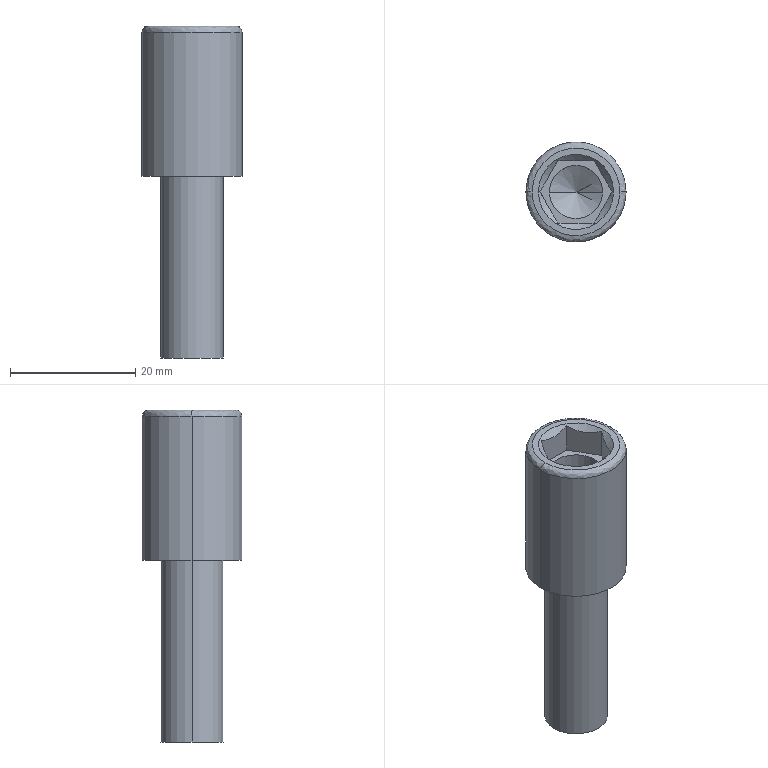Part | SolidWorks | features ICE 2, BaseBody 1 | 1 solid | 22 faces | box 16 x 16 x 53 mm | volume 5579 mm3 | plane 10 | cylinder 6 | cone 4 | spline 2 | commonest cylinder face diameters 8.5 x2 10 x2 16 x2
STEP:
#1=CARTESIAN_POINT('',(7.,0.,64.));
#2=VERTEX_POINT('',#1);
#3=CARTESIAN_POINT('',(-7.,0.,64.));
#4=VERTEX_POINT('',#3);
#5=CARTESIAN_POINT('',(7.,0.,64.));
#6=CARTESIAN_POINT('',(7.,-14.,64.));
#7=CARTESIAN_POINT('',(-7.,-14.,64.));
#8=CARTESIAN_POINT('',(-7.,0.,64.));
#9=(BOUNDED_CURVE()B_SPLINE_CURVE(3,(#5,#6,#7,#8),.UNSPECIFIED.,.F.,.F.)B_SPLINE_CURVE_WITH_KNOTS((4,4),(0.,1.),.UNSPECIFIED.)CURVE()GEOMETRIC_REPRESENTATION_ITEM()RATIONAL_B_SPLINE_CURVE((1.,0.3333,0.3333,1.))REPRESENTATION_ITEM(''));
#10=EDGE_CURVE('',#2,#4,#9,.T.);
#11=ORIENTED_EDGE('',*,*,#10,.T.);
#12=CARTESIAN_POINT('',(-8.,0.,63.));
#13=VERTEX_POINT('',#12);
#14=CARTESIAN_POINT('',(-7.,0.,63.));
#15=DIRECTION('',(0.,-1.,0.));
#16=DIRECTION('',(-1.,0.,0.));
#17=AXIS2_PLACEMENT_3D('',#14,#15,#16);
#18=CIRCLE('',#17,1.);
#19=EDGE_CURVE('',#4,#13,#18,.T.);
#20=ORIENTED_EDGE('',*,*,#19,.T.);
#21=CARTESIAN_POINT('',(8.,0.,63.));
#22=VERTEX_POINT('',#21);
#23=CARTESIAN_POINT('',(0.,0.,63.));
#24=DIRECTION('',(0.,0.,-1.));
#25=DIRECTION('',(-1.,0.,0.));
#26=AXIS2_PLACEMENT_3D('',#23,#24,#25);
#27=CIRCLE('',#26,8.);
#28=EDGE_CURVE('',#22,#13,#27,.T.);
#29=ORIENTED_EDGE('',*,*,#28,.F.);
#30=CARTESIAN_POINT('',(7.,0.,63.));
#31=DIRECTION('',(0.,1.,0.));
#32=DIRECTION('',(1.,0.,0.));
#33=AXIS2_PLACEMENT_3D('',#30,#31,#32);
#34=CIRCLE('',#33,1.);
#35=EDGE_CURVE('',#2,#22,#34,.T.);
#36=ORIENTED_EDGE('',*,*,#35,.F.);
#37=EDGE_LOOP('',(#11,#20,#29,#36));
#38=FACE_OUTER_BOUND('',#37,.T.);
#39=CARTESIAN_POINT('',(-7.,0.,64.));
#40=CARTESIAN_POINT('',(-7.,-14.,64.));
#41=CARTESIAN_POINT('',(7.,-14.,64.));
#42=CARTESIAN_POINT('',(7.,0.,64.));
#43=CARTESIAN_POINT('',(-7.586,0.,64.));
#44=CARTESIAN_POINT('',(-7.586,-15.172,64.));
#45=CARTESIAN_POINT('',(7.586,-15.172,64.));
#46=CARTESIAN_POINT('',(7.586,0.,64.));
#47=CARTESIAN_POINT('',(-8.,0.,63.586));
#48=CARTESIAN_POINT('',(-8.,-16.,63.586));
#49=CARTESIAN_POINT('',(8.,-16.,63.586));
#50=CARTESIAN_POINT('',(8.,0.,63.586));
#51=CARTESIAN_POINT('',(-8.,0.,63.));
#52=CARTESIAN_POINT('',(-8.,-16.,63.));
#53=CARTESIAN_POINT('',(8.,-16.,63.));
#54=CARTESIAN_POINT('',(8.,0.,63.));
#55=(BOUNDED_SURFACE()B_SPLINE_SURFACE(3,3,((#39,#40,#41,#42),(#43,#44,#45,#46),(#47,#48,#49,#50),(#51,#52,#53,#54)),.UNSPECIFIED.,.F.,.F.,.F.)B_SPLINE_SURFACE_WITH_KNOTS((4,4),(4,4),(0.,1.),(0.,1.),.UNSPECIFIED.)GEOMETRIC_REPRESENTATION_ITEM()RATIONAL_B_SPLINE_SURFACE(((1.,0.3333,0.3333,1.),(0.8047,0.2682,0.2682,0.8047),(0.8047,0.2682,0.2682,0.8047),(1.,0.3333,0.3333,1.)))REPRESENTATION_ITEM('')SURFACE());
#56=ADVANCED_FACE('',(#38),#55,.T.);
#57=CARTESIAN_POINT('',(-5.,0.,40.));
#58=VERTEX_POINT('',#57);
#59=CARTESIAN_POINT('',(5.,0.,40.));
#60=VERTEX_POINT('',#59);
#61=CARTESIAN_POINT('',(0.,0.,40.));
#62=DIRECTION('',(0.,0.,-1.));
#63=DIRECTION('',(-1.,0.,0.));
#64=AXIS2_PLACEMENT_3D('',#61,#62,#63);
#65=CIRCLE('',#64,5.);
#66=EDGE_CURVE('',#58,#60,#65,.T.);
#67=ORIENTED_EDGE('',*,*,#66,.T.);
#68=CARTESIAN_POINT('',(5.,0.,11.));
#69=VERTEX_POINT('',#68);
#70=CARTESIAN_POINT('',(5.,0.,37.));
#71=DIRECTION('',(0.,0.,-1.));
#72=VECTOR('',#71,1000.);
#73=LINE('',#70,#72);
#74=EDGE_CURVE('',#60,#69,#73,.T.);
#75=ORIENTED_EDGE('',*,*,#74,.T.);
#76=CARTESIAN_POINT('',(-5.,0.,11.));
#77=VERTEX_POINT('',#76);
#78=CARTESIAN_POINT('',(0.,0.,11.));
#79=DIRECTION('',(0.,0.,1.));
#80=DIRECTION('',(-1.,0.,0.));
#81=AXIS2_PLACEMENT_3D('',#78,#79,#80);
#82=CIRCLE('',#81,5.);
#83=EDGE_CURVE('',#69,#77,#82,.T.);
#84=ORIENTED_EDGE('',*,*,#83,.T.);
#85=CARTESIAN_POINT('',(-5.,0.,37.));
#86=DIRECTION('',(0.,0.,-1.));
#87=VECTOR('',#86,1000.);
#88=LINE('',#85,#87);
#89=EDGE_CURVE('',#58,#77,#88,.T.);
#90=ORIENTED_EDGE('',*,*,#89,.F.);
#91=EDGE_LOOP('',(#67,#75,#84,#90));
#92=FACE_OUTER_BOUND('',#91,.T.);
#93=CARTESIAN_POINT('',(0.,0.,37.));
#94=DIRECTION('',(0.,0.,-1.));
#95=DIRECTION('',(-1.,0.,0.));
#96=AXIS2_PLACEMENT_3D('',#93,#94,#95);
#97=CYLINDRICAL_SURFACE('',#96,5.);
#98=ADVANCED_FACE('',(#92),#97,.T.);
#99=CARTESIAN_POINT('',(-5.774,0.,63.774));
#100=VERTEX_POINT('',#99);
#101=CARTESIAN_POINT('',(-2.887,-5.,63.774));
#102=VERTEX_POINT('',#101);
#103=CARTESIAN_POINT('',(-5.774,0.,63.774));
#104=CARTESIAN_POINT('',(-5.548,-0.3907,63.548));
#105=CARTESIAN_POINT('',(-5.317,-0.7901,63.356));
#106=CARTESIAN_POINT('',(-4.959,-1.411,63.151));
#107=CARTESIAN_POINT('',(-4.837,-1.621,63.096));
#108=CARTESIAN_POINT('',(-4.589,-2.051,63.021));
#109=CARTESIAN_POINT('',(-4.461,-2.273,63.001));
#110=CARTESIAN_POINT('',(-4.083,-2.927,62.999));
#111=CARTESIAN_POINT('',(-3.836,-3.356,63.075));
#112=CARTESIAN_POINT('',(-3.347,-4.202,63.352));
#113=CARTESIAN_POINT('',(-3.114,-4.607,63.547));
#114=CARTESIAN_POINT('',(-2.887,-5.,63.774));
#115=B_SPLINE_CURVE_WITH_KNOTS('',3,(#103,#104,#105,#106,#107,#108,#109,#110,#111,#112,#113,#114),.UNSPECIFIED.,.F.,.F.,(4,2,2,2,2,4),(0.,0.001491,0.002236,0.002982,0.004473,0.005964),.UNSPECIFIED.);
#116=EDGE_CURVE('',#100,#102,#115,.T.);
#117=ORIENTED_EDGE('',*,*,#116,.F.);
#118=CARTESIAN_POINT('',(-6.,0.,64.));
#119=VERTEX_POINT('',#118);
#120=CARTESIAN_POINT('',(-6.,0.,64.));
#121=DIRECTION('',(-0.7071,0.,0.7071));
#122=VECTOR('',#121,1000.);
#123=LINE('',#120,#122);
#124=EDGE_CURVE('',#100,#119,#123,.T.);
#125=ORIENTED_EDGE('',*,*,#124,.T.);
#126=CARTESIAN_POINT('',(6.,0.,64.));
#127=VERTEX_POINT('',#126);
#128=CARTESIAN_POINT('',(0.,0.,64.));
#129=DIRECTION('',(0.,0.,-1.));
#130=DIRECTION('',(1.,0.,0.));
#131=AXIS2_PLACEMENT_3D('',#128,#129,#130);
#132=CIRCLE('',#131,6.);
#133=EDGE_CURVE('',#127,#119,#132,.T.);
#134=ORIENTED_EDGE('',*,*,#133,.F.);
#135=CARTESIAN_POINT('',(5.774,0.,63.774));
#136=VERTEX_POINT('',#135);
#137=CARTESIAN_POINT('',(6.,0.,64.));
#138=DIRECTION('',(0.7071,0.,0.7071));
#139=VECTOR('',#138,1000.);
#140=LINE('',#137,#139);
#141=EDGE_CURVE('',#136,#127,#140,.T.);
#142=ORIENTED_EDGE('',*,*,#141,.F.);
#143=CARTESIAN_POINT('',(2.887,-5.,63.774));
#144=VERTEX_POINT('',#143);
#145=CARTESIAN_POINT('',(2.887,-5.,63.774));
#146=CARTESIAN_POINT('',(3.112,-4.609,63.548));
#147=CARTESIAN_POINT('',(3.343,-4.21,63.356));
#148=CARTESIAN_POINT('',(3.701,-3.589,63.151));
#149=CARTESIAN_POINT('',(3.823,-3.379,63.096));
#150=CARTESIAN_POINT('',(4.071,-2.949,63.021));
#151=CARTESIAN_POINT('',(4.199,-2.727,63.001));
#152=CARTESIAN_POINT('',(4.577,-2.073,62.999));
#153=CARTESIAN_POINT('',(4.825,-1.644,63.075));
#154=CARTESIAN_POINT('',(5.313,-0.7976,63.352));
#155=CARTESIAN_POINT('',(5.547,-0.393,63.547));
#156=CARTESIAN_POINT('',(5.774,0.,63.774));
#157=B_SPLINE_CURVE_WITH_KNOTS('',3,(#145,#146,#147,#148,#149,#150,#151,#152,#153,#154,#155,#156),.UNSPECIFIED.,.F.,.F.,(4,2,2,2,2,4),(0.,0.001491,0.002236,0.002982,0.004473,0.005964),.UNSPECIFIED.);
#158=EDGE_CURVE('',#144,#136,#157,.T.);
#159=ORIENTED_EDGE('',*,*,#158,.F.);
#160=CARTESIAN_POINT('',(-2.887,-5.,63.774));
#161=CARTESIAN_POINT('',(-2.436,-5.,63.548));
#162=CARTESIAN_POINT('',(-1.974,-5.,63.356));
#163=CARTESIAN_POINT('',(-1.258,-5.,63.151));
#164=CARTESIAN_POINT('',(-1.015,-5.,63.096));
#165=CARTESIAN_POINT('',(-0.5183,-5.,63.021));
#166=CARTESIAN_POINT('',(-0.2626,-5.,63.001));
#167=CARTESIAN_POINT('',(0.4934,-5.,62.999));
#168=CARTESIAN_POINT('',(0.9888,-5.,63.075));
#169=CARTESIAN_POINT('',(1.966,-5.,63.352));
#170=CARTESIAN_POINT('',(2.433,-5.,63.547));
#171=CARTESIAN_POINT('',(2.887,-5.,63.774));
#172=B_SPLINE_CURVE_WITH_KNOTS('',3,(#160,#161,#162,#163,#164,#165,#166,#167,#168,#169,#170,#171),.UNSPECIFIED.,.F.,.F.,(4,2,2,2,2,4),(0.,0.001491,0.002236,0.002982,0.004473,0.005964),.UNSPECIFIED.);
#173=EDGE_CURVE('',#102,#144,#172,.T.);
#174=ORIENTED_EDGE('',*,*,#173,.F.);
#175=EDGE_LOOP('',(#117,#125,#134,#142,#159,#174));
#176=FACE_OUTER_BOUND('',#175,.T.);
#177=CARTESIAN_POINT('',(0.,0.,64.));
#178=DIRECTION('',(0.,0.,1.));
#179=DIRECTION('',(1.,0.,0.));
#180=AXIS2_PLACEMENT_3D('',#177,#178,#179);
#181=CONICAL_SURFACE('',#180,6.,0.7854);
#182=ADVANCED_FACE('',(#176),#181,.F.);
#183=CARTESIAN_POINT('',(-4.25,0.,41.));
#184=VERTEX_POINT('',#183);
#185=CARTESIAN_POINT('',(4.25,0.,41.));
#186=VERTEX_POINT('',#185);
#187=CARTESIAN_POINT('',(0.,0.,41.));
#188=DIRECTION('',(0.,0.,1.));
#189=DIRECTION('',(1.,0.,0.));
#190=AXIS2_PLACEMENT_3D('',#187,#188,#189);
#191=CIRCLE('',#190,4.25);
#192=EDGE_CURVE('',#184,#186,#191,.T.);
#193=ORIENTED_EDGE('',*,*,#192,.F.);
#194=CARTESIAN_POINT('',(-4.25,0.,59.));
#195=VERTEX_POINT('',#194);
#196=CARTESIAN_POINT('',(-4.25,0.,59.));
#197=DIRECTION('',(0.,0.,1.));
#198=VECTOR('',#197,1000.);
#199=LINE('',#196,#198);
#200=EDGE_CURVE('',#184,#195,#199,.T.);
#201=ORIENTED_EDGE('',*,*,#200,.T.);
#202=CARTESIAN_POINT('',(4.25,0.,59.));
#203=VERTEX_POINT('',#202);
#204=CARTESIAN_POINT('',(0.,0.,59.));
#205=DIRECTION('',(0.,0.,-1.));
#206=DIRECTION('',(1.,0.,0.));
#207=AXIS2_PLACEMENT_3D('',#204,#205,#206);
#208=CIRCLE('',#207,4.25);
#209=EDGE_CURVE('',#203,#195,#208,.T.);
#210=ORIENTED_EDGE('',*,*,#209,.F.);
#211=CARTESIAN_POINT('',(4.25,0.,59.));
#212=DIRECTION('',(0.,0.,1.));
#213=VECTOR('',#212,1000.);
#214=LINE('',#211,#213);
#215=EDGE_CURVE('',#186,#203,#214,.T.);
#216=ORIENTED_EDGE('',*,*,#215,.F.);
#217=EDGE_LOOP('',(#193,#201,#210,#216));
#218=FACE_OUTER_BOUND('',#217,.T.);
#219=CARTESIAN_POINT('',(0.,0.,59.));
#220=DIRECTION('',(0.,0.,1.));
#221=DIRECTION('',(1.,0.,0.));
#222=AXIS2_PLACEMENT_3D('',#219,#220,#221);
#223=CYLINDRICAL_SURFACE('',#222,4.25);
#224=ADVANCED_FACE('',(#218),#223,.F.);
#225=CARTESIAN_POINT('',(0.,0.,38.446));
#226=VERTEX_POINT('',#225);
#227=CARTESIAN_POINT('',(4.25,0.,41.));
#228=DIRECTION('',(0.8572,0.,0.515));
#229=VECTOR('',#228,1000.);
#230=LINE('',#227,#229);
#231=EDGE_CURVE('',#226,#186,#230,.T.);
#232=ORIENTED_EDGE('',*,*,#231,.F.);
#233=CARTESIAN_POINT('',(-4.25,0.,41.));
#234=DIRECTION('',(-0.8572,0.,0.515));
#235=VECTOR('',#234,1000.);
#236=LINE('',#233,#235);
#237=EDGE_CURVE('',#226,#184,#236,.T.);
#238=ORIENTED_EDGE('',*,*,#237,.T.);
#239=ORIENTED_EDGE('',*,*,#192,.T.);
#240=EDGE_LOOP('',(#232,#238,#239));
#241=FACE_OUTER_BOUND('',#240,.T.);
#242=CARTESIAN_POINT('',(0.,0.,41.));
#243=DIRECTION('',(0.,0.,1.));
#244=DIRECTION('',(1.,0.,0.));
#245=AXIS2_PLACEMENT_3D('',#242,#243,#244);
#246=CONICAL_SURFACE('',#245,4.25,1.03);
#247=ADVANCED_FACE('',(#241),#246,.F.);
#248=CARTESIAN_POINT('',(0.,0.,63.));
#249=DIRECTION('',(0.,0.,-1.));
#250=DIRECTION('',(-1.,0.,0.));
#251=AXIS2_PLACEMENT_3D('',#248,#249,#250);
#252=CIRCLE('',#251,8.);
#253=EDGE_CURVE('',#13,#22,#252,.T.);
#254=ORIENTED_EDGE('',*,*,#253,.T.);
#255=CARTESIAN_POINT('',(8.,0.,40.));
#256=VERTEX_POINT('',#255);
#257=CARTESIAN_POINT('',(8.,0.,64.));
#258=DIRECTION('',(0.,0.,-1.));
#259=VECTOR('',#258,1000.);
#260=LINE('',#257,#259);
#261=EDGE_CURVE('',#22,#256,#260,.T.);
#262=ORIENTED_EDGE('',*,*,#261,.T.);
#263=CARTESIAN_POINT('',(-8.,0.,40.));
#264=VERTEX_POINT('',#263);
#265=CARTESIAN_POINT('',(0.,0.,40.));
#266=DIRECTION('',(0.,0.,-1.));
#267=DIRECTION('',(-1.,0.,0.));
#268=AXIS2_PLACEMENT_3D('',#265,#266,#267);
#269=CIRCLE('',#268,8.);
#270=EDGE_CURVE('',#264,#256,#269,.T.);
#271=ORIENTED_EDGE('',*,*,#270,.F.);
#272=CARTESIAN_POINT('',(-8.,0.,64.));
#273=DIRECTION('',(0.,0.,-1.));
#274=VECTOR('',#273,1000.);
#275=LINE('',#272,#274);
#276=EDGE_CURVE('',#13,#264,#275,.T.);
#277=ORIENTED_EDGE('',*,*,#276,.F.);
#278=EDGE_LOOP('',(#254,#262,#271,#277));
#279=FACE_OUTER_BOUND('',#278,.T.);
#280=CARTESIAN_POINT('',(0.,0.,64.));
#281=DIRECTION('',(0.,0.,-1.));
#282=DIRECTION('',(-1.,0.,0.));
#283=AXIS2_PLACEMENT_3D('',#280,#281,#282);
#284=CYLINDRICAL_SURFACE('',#283,8.);
#285=ADVANCED_FACE('',(#279),#284,.T.);
#286=ORIENTED_EDGE('',*,*,#261,.F.);
#287=ORIENTED_EDGE('',*,*,#28,.T.);
#288=ORIENTED_EDGE('',*,*,#276,.T.);
#289=CARTESIAN_POINT('',(0.,0.,40.));
#290=DIRECTION('',(0.,0.,-1.));
#291=DIRECTION('',(-1.,0.,0.));
#292=AXIS2_PLACEMENT_3D('',#289,#290,#291);
#293=CIRCLE('',#292,8.);
#294=EDGE_CURVE('',#256,#264,#293,.T.);
#295=ORIENTED_EDGE('',*,*,#294,.F.);
#296=EDGE_LOOP('',(#286,#287,#288,#295));
#297=FACE_OUTER_BOUND('',#296,.T.);
#298=CARTESIAN_POINT('',(0.,0.,64.));
#299=DIRECTION('',(0.,0.,-1.));
#300=DIRECTION('',(-1.,0.,0.));
#301=AXIS2_PLACEMENT_3D('',#298,#299,#300);
#302=CYLINDRICAL_SURFACE('',#301,8.);
#303=ADVANCED_FACE('',(#297),#302,.T.);
#304=ORIENTED_EDGE('',*,*,#19,.F.);
#305=CARTESIAN_POINT('',(-7.,0.,64.));
#306=CARTESIAN_POINT('',(-7.,14.,64.));
#307=CARTESIAN_POINT('',(7.,14.,64.));
#308=CARTESIAN_POINT('',(7.,0.,64.));
#309=(BOUNDED_CURVE()B_SPLINE_CURVE(3,(#305,#306,#307,#308),.UNSPECIFIED.,.F.,.T.)B_SPLINE_CURVE_WITH_KNOTS((4,4),(0.,1.),.UNSPECIFIED.)CURVE()GEOMETRIC_REPRESENTATION_ITEM()RATIONAL_B_SPLINE_CURVE((1.,0.3333,0.3333,1.))REPRESENTATION_ITEM(''));
#310=EDGE_CURVE('',#4,#2,#309,.T.);
#311=ORIENTED_EDGE('',*,*,#310,.T.);
#312=ORIENTED_EDGE('',*,*,#35,.T.);
#313=ORIENTED_EDGE('',*,*,#253,.F.);
#314=EDGE_LOOP('',(#304,#311,#312,#313));
#315=FACE_OUTER_BOUND('',#314,.T.);
#316=CARTESIAN_POINT('',(7.,0.,64.));
#317=CARTESIAN_POINT('',(7.,14.,64.));
#318=CARTESIAN_POINT('',(-7.,14.,64.));
#319=CARTESIAN_POINT('',(-7.,0.,64.));
#320=CARTESIAN_POINT('',(7.586,0.,64.));
#321=CARTESIAN_POINT('',(7.586,15.172,64.));
#322=CARTESIAN_POINT('',(-7.586,15.172,64.));
#323=CARTESIAN_POINT('',(-7.586,0.,64.));
#324=CARTESIAN_POINT('',(8.,0.,63.586));
#325=CARTESIAN_POINT('',(8.,16.,63.586));
#326=CARTESIAN_POINT('',(-8.,16.,63.586));
#327=CARTESIAN_POINT('',(-8.,0.,63.586));
#328=CARTESIAN_POINT('',(8.,0.,63.));
#329=CARTESIAN_POINT('',(8.,16.,63.));
#330=CARTESIAN_POINT('',(-8.,16.,63.));
#331=CARTESIAN_POINT('',(-8.,0.,63.));
#332=(BOUNDED_SURFACE()B_SPLINE_SURFACE(3,3,((#316,#317,#318,#319),(#320,#321,#322,#323),(#324,#325,#326,#327),(#328,#329,#330,#331)),.UNSPECIFIED.,.F.,.F.,.T.)B_SPLINE_SURFACE_WITH_KNOTS((4,4),(4,4),(0.,1.),(0.,1.),.UNSPECIFIED.)GEOMETRIC_REPRESENTATION_ITEM()RATIONAL_B_SPLINE_SURFACE(((1.,0.3333,0.3333,1.),(0.8047,0.2682,0.2682,0.8047),(0.8047,0.2682,0.2682,0.8047),(1.,0.3333,0.3333,1.)))REPRESENTATION_ITEM('')SURFACE());
#333=ADVANCED_FACE('',(#315),#332,.T.);
#334=ORIENTED_EDGE('',*,*,#133,.T.);
#335=CARTESIAN_POINT('',(0.,0.,64.));
#336=DIRECTION('',(0.,0.,-1.));
#337=DIRECTION('',(1.,0.,0.));
#338=AXIS2_PLACEMENT_3D('',#335,#336,#337);
#339=CIRCLE('',#338,6.);
#340=EDGE_CURVE('',#119,#127,#339,.T.);
#341=ORIENTED_EDGE('',*,*,#340,.T.);
#342=EDGE_LOOP('',(#334,#341));
#343=FACE_BOUND('',#342,.T.);
#344=ORIENTED_EDGE('',*,*,#310,.F.);
#345=ORIENTED_EDGE('',*,*,#10,.F.);
#346=EDGE_LOOP('',(#344,#345));
#347=FACE_OUTER_BOUND('',#346,.T.);
#348=CARTESIAN_POINT('',(0.,0.,64.));
#349=DIRECTION('',(0.,0.,1.));
#350=DIRECTION('',(1.,0.,0.));
#351=AXIS2_PLACEMENT_3D('',#348,#349,#350);
#352=PLANE('',#351);
#353=ADVANCED_FACE('',(#343,#347),#352,.T.);
#354=ORIENTED_EDGE('',*,*,#124,.F.);
#355=CARTESIAN_POINT('',(-2.887,5.,63.774));
#356=VERTEX_POINT('',#355);
#357=CARTESIAN_POINT('',(-2.887,5.,63.774));
#358=CARTESIAN_POINT('',(-3.112,4.609,63.548));
#359=CARTESIAN_POINT('',(-3.343,4.21,63.356));
#360=CARTESIAN_POINT('',(-3.701,3.589,63.151));
#361=CARTESIAN_POINT('',(-3.823,3.379,63.096));
#362=CARTESIAN_POINT('',(-4.071,2.949,63.021));
#363=CARTESIAN_POINT('',(-4.199,2.727,63.001));
#364=CARTESIAN_POINT('',(-4.577,2.073,62.999));
#365=CARTESIAN_POINT('',(-4.825,1.644,63.075));
#366=CARTESIAN_POINT('',(-5.313,0.7976,63.352));
#367=CARTESIAN_POINT('',(-5.547,0.393,63.547));
#368=CARTESIAN_POINT('',(-5.774,0.,63.774));
#369=B_SPLINE_CURVE_WITH_KNOTS('',3,(#357,#358,#359,#360,#361,#362,#363,#364,#365,#366,#367,#368),.UNSPECIFIED.,.F.,.F.,(4,2,2,2,2,4),(0.,0.001491,0.002236,0.002982,0.004473,0.005964),.UNSPECIFIED.);
#370=EDGE_CURVE('',#356,#100,#369,.T.);
#371=ORIENTED_EDGE('',*,*,#370,.F.);
#372=CARTESIAN_POINT('',(2.887,5.,63.774));
#373=VERTEX_POINT('',#372);
#374=CARTESIAN_POINT('',(2.887,5.,63.774));
#375=CARTESIAN_POINT('',(2.436,5.,63.548));
#376=CARTESIAN_POINT('',(1.974,5.,63.356));
#377=CARTESIAN_POINT('',(1.258,5.,63.151));
#378=CARTESIAN_POINT('',(1.015,5.,63.096));
#379=CARTESIAN_POINT('',(0.5183,5.,63.021));
#380=CARTESIAN_POINT('',(0.2626,5.,63.001));
#381=CARTESIAN_POINT('',(-0.4934,5.,62.999));
#382=CARTESIAN_POINT('',(-0.9888,5.,63.075));
#383=CARTESIAN_POINT('',(-1.966,5.,63.352));
#384=CARTESIAN_POINT('',(-2.433,5.,63.547));
#385=CARTESIAN_POINT('',(-2.887,5.,63.774));
#386=B_SPLINE_CURVE_WITH_KNOTS('',3,(#374,#375,#376,#377,#378,#379,#380,#381,#382,#383,#384,#385),.UNSPECIFIED.,.F.,.F.,(4,2,2,2,2,4),(0.,0.001491,0.002236,0.002982,0.004473,0.005964),.UNSPECIFIED.);
#387=EDGE_CURVE('',#373,#356,#386,.T.);
#388=ORIENTED_EDGE('',*,*,#387,.F.);
#389=CARTESIAN_POINT('',(5.774,0.,63.774));
#390=CARTESIAN_POINT('',(5.548,0.3907,63.548));
#391=CARTESIAN_POINT('',(5.317,0.7901,63.356));
#392=CARTESIAN_POINT('',(4.959,1.411,63.151));
#393=CARTESIAN_POINT('',(4.837,1.621,63.096));
#394=CARTESIAN_POINT('',(4.589,2.051,63.021));
#395=CARTESIAN_POINT('',(4.461,2.273,63.001));
#396=CARTESIAN_POINT('',(4.083,2.927,62.999));
#397=CARTESIAN_POINT('',(3.836,3.356,63.075));
#398=CARTESIAN_POINT('',(3.347,4.202,63.352));
#399=CARTESIAN_POINT('',(3.114,4.607,63.547));
#400=CARTESIAN_POINT('',(2.887,5.,63.774));
#401=B_SPLINE_CURVE_WITH_KNOTS('',3,(#389,#390,#391,#392,#393,#394,#395,#396,#397,#398,#399,#400),.UNSPECIFIED.,.F.,.F.,(4,2,2,2,2,4),(0.,0.001491,0.002236,0.002982,0.004473,0.005964),.UNSPECIFIED.);
#402=EDGE_CURVE('',#136,#373,#401,.T.);
#403=ORIENTED_EDGE('',*,*,#402,.F.);
#404=ORIENTED_EDGE('',*,*,#141,.T.);
#405=ORIENTED_EDGE('',*,*,#340,.F.);
#406=EDGE_LOOP('',(#354,#371,#388,#403,#404,#405));
#407=FACE_OUTER_BOUND('',#406,.T.);
#408=CARTESIAN_POINT('',(0.,0.,64.));
#409=DIRECTION('',(0.,0.,1.));
#410=DIRECTION('',(1.,0.,0.));
#411=AXIS2_PLACEMENT_3D('',#408,#409,#410);
#412=CONICAL_SURFACE('',#411,6.,0.7854);
#413=ADVANCED_FACE('',(#407),#412,.F.);
#414=CARTESIAN_POINT('',(-5.774,0.,59.));
#415=VERTEX_POINT('',#414);
#416=CARTESIAN_POINT('',(-5.774,0.,59.));
#417=DIRECTION('',(0.,0.,1.));
#418=VECTOR('',#417,1000.);
#419=LINE('',#416,#418);
#420=EDGE_CURVE('',#415,#100,#419,.T.);
#421=ORIENTED_EDGE('',*,*,#420,.F.);
#422=CARTESIAN_POINT('',(-2.887,5.,59.));
#423=VERTEX_POINT('',#422);
#424=CARTESIAN_POINT('',(-2.887,5.,59.));
#425=DIRECTION('',(-0.5,-0.866,0.));
#426=VECTOR('',#425,1000.);
#427=LINE('',#424,#426);
#428=EDGE_CURVE('',#423,#415,#427,.T.);
#429=ORIENTED_EDGE('',*,*,#428,.F.);
#430=CARTESIAN_POINT('',(-2.887,5.,59.));
#431=DIRECTION('',(0.,0.,-1.));
#432=VECTOR('',#431,1000.);
#433=LINE('',#430,#432);
#434=EDGE_CURVE('',#356,#423,#433,.T.);
#435=ORIENTED_EDGE('',*,*,#434,.F.);
#436=ORIENTED_EDGE('',*,*,#370,.T.);
#437=EDGE_LOOP('',(#421,#429,#435,#436));
#438=FACE_OUTER_BOUND('',#437,.T.);
#439=CARTESIAN_POINT('',(-2.887,5.,59.));
#440=DIRECTION('',(-0.866,0.5,0.));
#441=DIRECTION('',(-0.5,-0.866,0.));
#442=AXIS2_PLACEMENT_3D('',#439,#440,#441);
#443=PLANE('',#442);
#444=ADVANCED_FACE('',(#438),#443,.F.);
#445=ORIENTED_EDGE('',*,*,#434,.T.);
#446=CARTESIAN_POINT('',(2.887,5.,59.));
#447=VERTEX_POINT('',#446);
#448=CARTESIAN_POINT('',(2.887,5.,59.));
#449=DIRECTION('',(-1.,0.,0.));
#450=VECTOR('',#449,1000.);
#451=LINE('',#448,#450);
#452=EDGE_CURVE('',#447,#423,#451,.T.);
#453=ORIENTED_EDGE('',*,*,#452,.F.);
#454=CARTESIAN_POINT('',(2.887,5.,59.));
#455=DIRECTION('',(0.,0.,-1.));
#456=VECTOR('',#455,1000.);
#457=LINE('',#454,#456);
#458=EDGE_CURVE('',#373,#447,#457,.T.);
#459=ORIENTED_EDGE('',*,*,#458,.F.);
#460=ORIENTED_EDGE('',*,*,#387,.T.);
#461=EDGE_LOOP('',(#445,#453,#459,#460));
#462=FACE_OUTER_BOUND('',#461,.T.);
#463=CARTESIAN_POINT('',(2.887,5.,59.));
#464=DIRECTION('',(0.,1.,0.));
#465=DIRECTION('',(-1.,0.,0.));
#466=AXIS2_PLACEMENT_3D('',#463,#464,#465);
#467=PLANE('',#466);
#468=ADVANCED_FACE('',(#462),#467,.F.);
#469=ORIENTED_EDGE('',*,*,#458,.T.);
#470=CARTESIAN_POINT('',(5.774,0.,59.));
#471=VERTEX_POINT('',#470);
#472=CARTESIAN_POINT('',(5.774,0.,59.));
#473=DIRECTION('',(-0.5,0.866,0.));
#474=VECTOR('',#473,1000.);
#475=LINE('',#472,#474);
#476=EDGE_CURVE('',#471,#447,#475,.T.);
#477=ORIENTED_EDGE('',*,*,#476,.F.);
#478=CARTESIAN_POINT('',(5.774,0.,59.));
#479=DIRECTION('',(0.,0.,-1.));
#480=VECTOR('',#479,1000.);
#481=LINE('',#478,#480);
#482=EDGE_CURVE('',#136,#471,#481,.T.);
#483=ORIENTED_EDGE('',*,*,#482,.F.);
#484=ORIENTED_EDGE('',*,*,#402,.T.);
#485=EDGE_LOOP('',(#469,#477,#483,#484));
#486=FACE_OUTER_BOUND('',#485,.T.);
#487=CARTESIAN_POINT('',(5.774,0.,59.));
#488=DIRECTION('',(0.866,0.5,0.));
#489=DIRECTION('',(-0.5,0.866,0.));
#490=AXIS2_PLACEMENT_3D('',#487,#488,#489);
#491=PLANE('',#490);
#492=ADVANCED_FACE('',(#486),#491,.F.);
#493=CARTESIAN_POINT('',(-2.887,-5.,59.));
#494=VERTEX_POINT('',#493);
#495=CARTESIAN_POINT('',(-2.887,-5.,59.));
#496=DIRECTION('',(0.,0.,1.));
#497=VECTOR('',#496,1000.);
#498=LINE('',#495,#497);
#499=EDGE_CURVE('',#494,#102,#498,.T.);
#500=ORIENTED_EDGE('',*,*,#499,.F.);
#501=CARTESIAN_POINT('',(-5.774,0.,59.));
#502=DIRECTION('',(0.5,-0.866,0.));
#503=VECTOR('',#502,1000.);
#504=LINE('',#501,#503);
#505=EDGE_CURVE('',#415,#494,#504,.T.);
#506=ORIENTED_EDGE('',*,*,#505,.F.);
#507=ORIENTED_EDGE('',*,*,#420,.T.);
#508=ORIENTED_EDGE('',*,*,#116,.T.);
#509=EDGE_LOOP('',(#500,#506,#507,#508));
#510=FACE_OUTER_BOUND('',#509,.T.);
#511=CARTESIAN_POINT('',(-5.774,0.,59.));
#512=DIRECTION('',(-0.866,-0.5,0.));
#513=DIRECTION('',(0.5,-0.866,0.));
#514=AXIS2_PLACEMENT_3D('',#511,#512,#513);
#515=PLANE('',#514);
#516=ADVANCED_FACE('',(#510),#515,.F.);
#517=ORIENTED_EDGE('',*,*,#482,.T.);
#518=CARTESIAN_POINT('',(2.887,-5.,59.));
#519=VERTEX_POINT('',#518);
#520=CARTESIAN_POINT('',(2.887,-5.,59.));
#521=DIRECTION('',(0.5,0.866,0.));
#522=VECTOR('',#521,1000.);
#523=LINE('',#520,#522);
#524=EDGE_CURVE('',#519,#471,#523,.T.);
#525=ORIENTED_EDGE('',*,*,#524,.F.);
#526=CARTESIAN_POINT('',(2.887,-5.,59.));
#527=DIRECTION('',(0.,0.,-1.));
#528=VECTOR('',#527,1000.);
#529=LINE('',#526,#528);
#530=EDGE_CURVE('',#144,#519,#529,.T.);
#531=ORIENTED_EDGE('',*,*,#530,.F.);
#532=ORIENTED_EDGE('',*,*,#158,.T.);
#533=EDGE_LOOP('',(#517,#525,#531,#532));
#534=FACE_OUTER_BOUND('',#533,.T.);
#535=CARTESIAN_POINT('',(2.887,-5.,59.));
#536=DIRECTION('',(0.866,-0.5,0.));
#537=DIRECTION('',(0.5,0.866,0.));
#538=AXIS2_PLACEMENT_3D('',#535,#536,#537);
#539=PLANE('',#538);
#540=ADVANCED_FACE('',(#534),#539,.F.);
#541=ORIENTED_EDGE('',*,*,#530,.T.);
#542=CARTESIAN_POINT('',(-2.887,-5.,59.));
#543=DIRECTION('',(1.,0.,0.));
#544=VECTOR('',#543,1000.);
#545=LINE('',#542,#544);
#546=EDGE_CURVE('',#494,#519,#545,.T.);
#547=ORIENTED_EDGE('',*,*,#546,.F.);
#548=ORIENTED_EDGE('',*,*,#499,.T.);
#549=ORIENTED_EDGE('',*,*,#173,.T.);
#550=EDGE_LOOP('',(#541,#547,#548,#549));
#551=FACE_OUTER_BOUND('',#550,.T.);
#552=CARTESIAN_POINT('',(-2.887,-5.,59.));
#553=DIRECTION('',(0.,-1.,0.));
#554=DIRECTION('',(1.,0.,0.));
#555=AXIS2_PLACEMENT_3D('',#552,#553,#554);
#556=PLANE('',#555);
#557=ADVANCED_FACE('',(#551),#556,.F.);
#558=ORIENTED_EDGE('',*,*,#476,.T.);
#559=ORIENTED_EDGE('',*,*,#452,.T.);
#560=ORIENTED_EDGE('',*,*,#428,.T.);
#561=ORIENTED_EDGE('',*,*,#505,.T.);
#562=ORIENTED_EDGE('',*,*,#546,.T.);
#563=ORIENTED_EDGE('',*,*,#524,.T.);
#564=EDGE_LOOP('',(#558,#559,#560,#561,#562,#563));
#565=FACE_OUTER_BOUND('',#564,.T.);
#566=ORIENTED_EDGE('',*,*,#209,.T.);
#567=CARTESIAN_POINT('',(0.,0.,59.));
#568=DIRECTION('',(0.,0.,-1.));
#569=DIRECTION('',(1.,0.,0.));
#570=AXIS2_PLACEMENT_3D('',#567,#568,#569);
#571=CIRCLE('',#570,4.25);
#572=EDGE_CURVE('',#195,#203,#571,.T.);
#573=ORIENTED_EDGE('',*,*,#572,.T.);
#574=EDGE_LOOP('',(#566,#573));
#575=FACE_BOUND('',#574,.T.);
#576=CARTESIAN_POINT('',(0.,0.,59.));
#577=DIRECTION('',(0.,0.,1.));
#578=DIRECTION('',(1.,0.,0.));
#579=AXIS2_PLACEMENT_3D('',#576,#577,#578);
#580=PLANE('',#579);
#581=ADVANCED_FACE('',(#565,#575),#580,.T.);
#582=ORIENTED_EDGE('',*,*,#200,.F.);
#583=CARTESIAN_POINT('',(0.,0.,41.));
#584=DIRECTION('',(0.,0.,1.));
#585=DIRECTION('',(1.,0.,0.));
#586=AXIS2_PLACEMENT_3D('',#583,#584,#585);
#587=CIRCLE('',#586,4.25);
#588=EDGE_CURVE('',#186,#184,#587,.T.);
#589=ORIENTED_EDGE('',*,*,#588,.F.);
#590=ORIENTED_EDGE('',*,*,#215,.T.);
#591=ORIENTED_EDGE('',*,*,#572,.F.);
#592=EDGE_LOOP('',(#582,#589,#590,#591));
#593=FACE_OUTER_BOUND('',#592,.T.);
#594=CARTESIAN_POINT('',(0.,0.,59.));
#595=DIRECTION('',(0.,0.,1.));
#596=DIRECTION('',(1.,0.,0.));
#597=AXIS2_PLACEMENT_3D('',#594,#595,#596);
#598=CYLINDRICAL_SURFACE('',#597,4.25);
#599=ADVANCED_FACE('',(#593),#598,.F.);
#600=ORIENTED_EDGE('',*,*,#237,.F.);
#601=ORIENTED_EDGE('',*,*,#231,.T.);
#602=ORIENTED_EDGE('',*,*,#588,.T.);
#603=EDGE_LOOP('',(#600,#601,#602));
#604=FACE_OUTER_BOUND('',#603,.T.);
#605=CARTESIAN_POINT('',(0.,0.,41.));
#606=DIRECTION('',(0.,0.,1.));
#607=DIRECTION('',(1.,0.,0.));
#608=AXIS2_PLACEMENT_3D('',#605,#606,#607);
#609=CONICAL_SURFACE('',#608,4.25,1.03);
#610=ADVANCED_FACE('',(#604),#609,.F.);
#611=ORIENTED_EDGE('',*,*,#66,.F.);
#612=CARTESIAN_POINT('',(0.,0.,40.));
#613=DIRECTION('',(0.,0.,-1.));
#614=DIRECTION('',(-1.,0.,0.));
#615=AXIS2_PLACEMENT_3D('',#612,#613,#614);
#616=CIRCLE('',#615,5.);
#617=EDGE_CURVE('',#60,#58,#616,.T.);
#618=ORIENTED_EDGE('',*,*,#617,.F.);
#619=EDGE_LOOP('',(#611,#618));
#620=FACE_BOUND('',#619,.T.);
#621=ORIENTED_EDGE('',*,*,#270,.T.);
#622=ORIENTED_EDGE('',*,*,#294,.T.);
#623=EDGE_LOOP('',(#621,#622));
#624=FACE_OUTER_BOUND('',#623,.T.);
#625=CARTESIAN_POINT('',(0.,0.,40.));
#626=DIRECTION('',(0.,0.,-1.));
#627=DIRECTION('',(-1.,0.,0.));
#628=AXIS2_PLACEMENT_3D('',#625,#626,#627);
#629=PLANE('',#628);
#630=ADVANCED_FACE('',(#620,#624),#629,.T.);
#631=CARTESIAN_POINT('',(0.,0.,11.));
#632=DIRECTION('',(0.,0.,1.));
#633=DIRECTION('',(-1.,0.,0.));
#634=AXIS2_PLACEMENT_3D('',#631,#632,#633);
#635=CIRCLE('',#634,5.);
#636=EDGE_CURVE('',#77,#69,#635,.T.);
#637=ORIENTED_EDGE('',*,*,#636,.F.);
#638=ORIENTED_EDGE('',*,*,#83,.F.);
#639=EDGE_LOOP('',(#637,#638));
#640=FACE_OUTER_BOUND('',#639,.T.);
#641=CARTESIAN_POINT('',(0.,0.,11.));
#642=DIRECTION('',(0.,0.,-1.));
#643=DIRECTION('',(-1.,0.,0.));
#644=AXIS2_PLACEMENT_3D('',#641,#642,#643);
#645=PLANE('',#644);
#646=ADVANCED_FACE('',(#640),#645,.T.);
#647=ORIENTED_EDGE('',*,*,#74,.F.);
#648=ORIENTED_EDGE('',*,*,#617,.T.);
#649=ORIENTED_EDGE('',*,*,#89,.T.);
#650=ORIENTED_EDGE('',*,*,#636,.T.);
#651=EDGE_LOOP('',(#647,#648,#649,#650));
#652=FACE_OUTER_BOUND('',#651,.T.);
#653=CARTESIAN_POINT('',(0.,0.,37.));
#654=DIRECTION('',(0.,0.,-1.));
#655=DIRECTION('',(-1.,0.,0.));
#656=AXIS2_PLACEMENT_3D('',#653,#654,#655);
#657=CYLINDRICAL_SURFACE('',#656,5.);
#658=ADVANCED_FACE('',(#652),#657,.T.);
#659=CLOSED_SHELL('',(#56,#98,#182,#224,#247,#285,#303,#333,#353,#413,#444,#468,#492,#516,#540,#557,#581,#599,#610,#630,#646,#658));
#660=MANIFOLD_SOLID_BREP('',#659);
#661=CARTESIAN_POINT('',(0.,0.,0.));
#662=DIRECTION('',(0.,0.,1.));
#663=DIRECTION('',(1.,0.,0.));
#664=AXIS2_PLACEMENT_3D('',#661,#662,#663);
#665=(LENGTH_UNIT()NAMED_UNIT(*)SI_UNIT(.MILLI.,.METRE.));
#666=UNCERTAINTY_MEASURE_WITH_UNIT(LENGTH_MEASURE(0.00001),#665,'','');
#667=(NAMED_UNIT(*)PLANE_ANGLE_UNIT()SI_UNIT($,.RADIAN.));
#668=(NAMED_UNIT(*)SI_UNIT($,.STERADIAN.)SOLID_ANGLE_UNIT());
#669=(GEOMETRIC_REPRESENTATION_CONTEXT(3)GLOBAL_UNCERTAINTY_ASSIGNED_CONTEXT((#666))GLOBAL_UNIT_ASSIGNED_CONTEXT((#665,#667,#668))REPRESENTATION_CONTEXT('',''));
#670=ADVANCED_BREP_SHAPE_REPRESENTATION('',(#660,#664),#669);